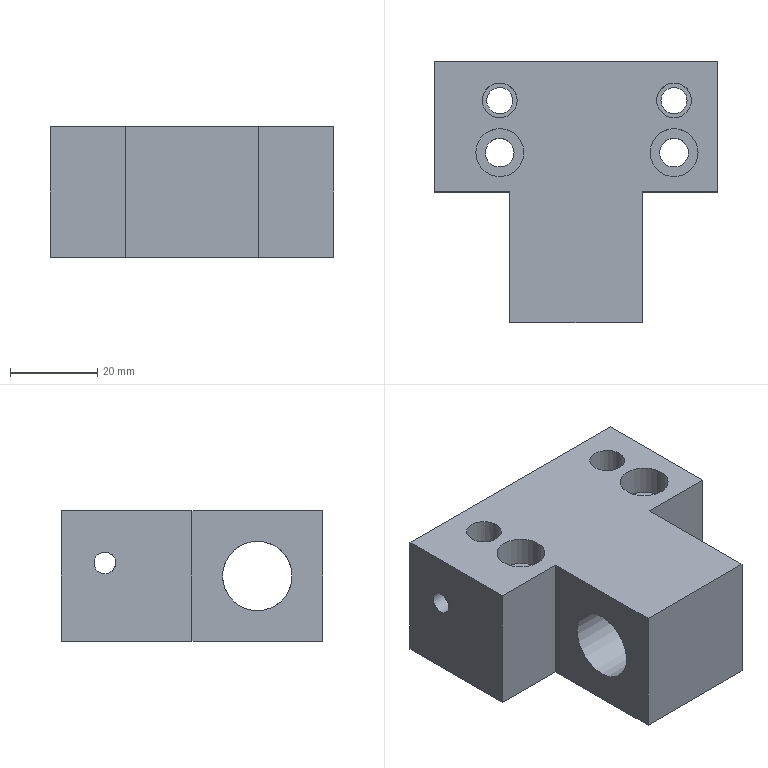Part | NX | features 5003_207_Bracket 2 | 1 solid | 26 faces | box 65 x 60 x 30 mm | volume 73364 mm3 | plane 14 | cylinder 12 | commonest cylinder face diameters 5 x3 6 x2 6.6 x2 8 x2 11 x2 16 x1
STEP:
#1=CARTESIAN_POINT('',(109.6,-462.,-238.));
#2=VERTEX_POINT('',#1);
#3=CARTESIAN_POINT('',(44.6,-462.,-238.));
#4=VERTEX_POINT('',#3);
#5=CARTESIAN_POINT('',(44.6,-462.,-238.));
#6=DIRECTION('',(-1.,0.,0.));
#7=VECTOR('',#6,1000.);
#8=LINE('',#5,#7);
#9=EDGE_CURVE('',#2,#4,#8,.T.);
#10=ORIENTED_EDGE('',*,*,#9,.T.);
#11=CARTESIAN_POINT('',(44.6,-462.,-208.));
#12=VERTEX_POINT('',#11);
#13=CARTESIAN_POINT('',(44.6,-462.,-208.));
#14=DIRECTION('',(0.,0.,-1.));
#15=VECTOR('',#14,1000.);
#16=LINE('',#13,#15);
#17=EDGE_CURVE('',#12,#4,#16,.T.);
#18=ORIENTED_EDGE('',*,*,#17,.F.);
#19=CARTESIAN_POINT('',(109.6,-462.,-208.));
#20=VERTEX_POINT('',#19);
#21=CARTESIAN_POINT('',(44.6,-462.,-208.));
#22=DIRECTION('',(-1.,0.,0.));
#23=VECTOR('',#22,1000.);
#24=LINE('',#21,#23);
#25=EDGE_CURVE('',#20,#12,#24,.T.);
#26=ORIENTED_EDGE('',*,*,#25,.F.);
#27=CARTESIAN_POINT('',(109.6,-462.,-208.));
#28=DIRECTION('',(0.,0.,-1.));
#29=VECTOR('',#28,1000.);
#30=LINE('',#27,#29);
#31=EDGE_CURVE('',#20,#2,#30,.T.);
#32=ORIENTED_EDGE('',*,*,#31,.T.);
#33=EDGE_LOOP('',(#10,#18,#26,#32));
#34=FACE_BOUND('',#33,.T.);
#35=CARTESIAN_POINT('',(44.6,-462.,-208.));
#36=DIRECTION('',(0.,-1.,0.));
#37=DIRECTION('',(1.,0.,0.));
#38=AXIS2_PLACEMENT_3D('',#35,#36,#37);
#39=PLANE('',#38);
#40=ADVANCED_FACE('',(#34),#39,.F.);
#41=CARTESIAN_POINT('',(44.6,-472.,-222.5));
#42=VERTEX_POINT('',#41);
#43=CARTESIAN_POINT('',(44.6,-472.,-220.));
#44=DIRECTION('',(-1.,0.,0.));
#45=DIRECTION('',(0.,0.,-1.));
#46=AXIS2_PLACEMENT_3D('',#43,#44,#45);
#47=CIRCLE('',#46,2.5);
#48=EDGE_CURVE('',#42,#42,#47,.T.);
#49=ORIENTED_EDGE('',*,*,#48,.F.);
#50=EDGE_LOOP('',(#49));
#51=FACE_BOUND('',#50,.T.);
#52=CARTESIAN_POINT('',(44.6,-492.,-238.));
#53=VERTEX_POINT('',#52);
#54=CARTESIAN_POINT('',(44.6,-492.,-238.));
#55=DIRECTION('',(0.,-1.,0.));
#56=VECTOR('',#55,1000.);
#57=LINE('',#54,#56);
#58=EDGE_CURVE('',#4,#53,#57,.T.);
#59=ORIENTED_EDGE('',*,*,#58,.T.);
#60=CARTESIAN_POINT('',(44.6,-492.,-208.));
#61=VERTEX_POINT('',#60);
#62=CARTESIAN_POINT('',(44.6,-492.,-208.));
#63=DIRECTION('',(0.,0.,-1.));
#64=VECTOR('',#63,1000.);
#65=LINE('',#62,#64);
#66=EDGE_CURVE('',#61,#53,#65,.T.);
#67=ORIENTED_EDGE('',*,*,#66,.F.);
#68=CARTESIAN_POINT('',(44.6,-492.,-208.));
#69=DIRECTION('',(0.,-1.,0.));
#70=VECTOR('',#69,1000.);
#71=LINE('',#68,#70);
#72=EDGE_CURVE('',#12,#61,#71,.T.);
#73=ORIENTED_EDGE('',*,*,#72,.F.);
#74=ORIENTED_EDGE('',*,*,#17,.T.);
#75=EDGE_LOOP('',(#59,#67,#73,#74));
#76=FACE_BOUND('',#75,.T.);
#77=CARTESIAN_POINT('',(44.6,-492.,-208.));
#78=DIRECTION('',(1.,0.,0.));
#79=DIRECTION('',(0.,0.,1.));
#80=AXIS2_PLACEMENT_3D('',#77,#78,#79);
#81=PLANE('',#80);
#82=ADVANCED_FACE('',(#51,#76),#81,.F.);
#83=CARTESIAN_POINT('',(61.855,-492.,-238.));
#84=VERTEX_POINT('',#83);
#85=CARTESIAN_POINT('',(61.855,-492.,-238.));
#86=DIRECTION('',(1.,0.,0.));
#87=VECTOR('',#86,1000.);
#88=LINE('',#85,#87);
#89=EDGE_CURVE('',#53,#84,#88,.T.);
#90=ORIENTED_EDGE('',*,*,#89,.T.);
#91=CARTESIAN_POINT('',(61.855,-492.,-208.));
#92=VERTEX_POINT('',#91);
#93=CARTESIAN_POINT('',(61.855,-492.,-208.));
#94=DIRECTION('',(0.,0.,-1.));
#95=VECTOR('',#94,1000.);
#96=LINE('',#93,#95);
#97=EDGE_CURVE('',#92,#84,#96,.T.);
#98=ORIENTED_EDGE('',*,*,#97,.F.);
#99=CARTESIAN_POINT('',(61.855,-492.,-208.));
#100=DIRECTION('',(1.,0.,0.));
#101=VECTOR('',#100,1000.);
#102=LINE('',#99,#101);
#103=EDGE_CURVE('',#61,#92,#102,.T.);
#104=ORIENTED_EDGE('',*,*,#103,.F.);
#105=ORIENTED_EDGE('',*,*,#66,.T.);
#106=EDGE_LOOP('',(#90,#98,#104,#105));
#107=FACE_BOUND('',#106,.T.);
#108=CARTESIAN_POINT('',(61.855,-492.,-208.));
#109=DIRECTION('',(0.,1.,0.));
#110=DIRECTION('',(-1.,0.,0.));
#111=AXIS2_PLACEMENT_3D('',#108,#109,#110);
#112=PLANE('',#111);
#113=ADVANCED_FACE('',(#107),#112,.F.);
#114=CARTESIAN_POINT('',(61.855,-507.,-231.));
#115=VERTEX_POINT('',#114);
#116=CARTESIAN_POINT('',(61.855,-507.,-223.));
#117=DIRECTION('',(-1.,0.,0.));
#118=DIRECTION('',(0.,0.,-1.));
#119=AXIS2_PLACEMENT_3D('',#116,#117,#118);
#120=CIRCLE('',#119,8.);
#121=EDGE_CURVE('',#115,#115,#120,.T.);
#122=ORIENTED_EDGE('',*,*,#121,.F.);
#123=EDGE_LOOP('',(#122));
#124=FACE_BOUND('',#123,.T.);
#125=CARTESIAN_POINT('',(61.855,-522.,-238.));
#126=VERTEX_POINT('',#125);
#127=CARTESIAN_POINT('',(61.855,-522.,-238.));
#128=DIRECTION('',(0.,-1.,0.));
#129=VECTOR('',#128,1000.);
#130=LINE('',#127,#129);
#131=EDGE_CURVE('',#84,#126,#130,.T.);
#132=ORIENTED_EDGE('',*,*,#131,.T.);
#133=CARTESIAN_POINT('',(61.855,-522.,-208.));
#134=VERTEX_POINT('',#133);
#135=CARTESIAN_POINT('',(61.855,-522.,-208.));
#136=DIRECTION('',(0.,0.,-1.));
#137=VECTOR('',#136,1000.);
#138=LINE('',#135,#137);
#139=EDGE_CURVE('',#134,#126,#138,.T.);
#140=ORIENTED_EDGE('',*,*,#139,.F.);
#141=CARTESIAN_POINT('',(61.855,-522.,-208.));
#142=DIRECTION('',(0.,-1.,0.));
#143=VECTOR('',#142,1000.);
#144=LINE('',#141,#143);
#145=EDGE_CURVE('',#92,#134,#144,.T.);
#146=ORIENTED_EDGE('',*,*,#145,.F.);
#147=ORIENTED_EDGE('',*,*,#97,.T.);
#148=EDGE_LOOP('',(#132,#140,#146,#147));
#149=FACE_BOUND('',#148,.T.);
#150=CARTESIAN_POINT('',(61.855,-522.,-208.));
#151=DIRECTION('',(1.,0.,0.));
#152=DIRECTION('',(0.,0.,1.));
#153=AXIS2_PLACEMENT_3D('',#150,#151,#152);
#154=PLANE('',#153);
#155=ADVANCED_FACE('',(#124,#149),#154,.F.);
#156=CARTESIAN_POINT('',(92.345,-522.,-238.));
#157=VERTEX_POINT('',#156);
#158=CARTESIAN_POINT('',(92.345,-522.,-238.));
#159=DIRECTION('',(1.,0.,0.));
#160=VECTOR('',#159,1000.);
#161=LINE('',#158,#160);
#162=EDGE_CURVE('',#126,#157,#161,.T.);
#163=ORIENTED_EDGE('',*,*,#162,.T.);
#164=CARTESIAN_POINT('',(92.345,-522.,-208.));
#165=VERTEX_POINT('',#164);
#166=CARTESIAN_POINT('',(92.345,-522.,-208.));
#167=DIRECTION('',(0.,0.,-1.));
#168=VECTOR('',#167,1000.);
#169=LINE('',#166,#168);
#170=EDGE_CURVE('',#165,#157,#169,.T.);
#171=ORIENTED_EDGE('',*,*,#170,.F.);
#172=CARTESIAN_POINT('',(92.345,-522.,-208.));
#173=DIRECTION('',(1.,0.,0.));
#174=VECTOR('',#173,1000.);
#175=LINE('',#172,#174);
#176=EDGE_CURVE('',#134,#165,#175,.T.);
#177=ORIENTED_EDGE('',*,*,#176,.F.);
#178=ORIENTED_EDGE('',*,*,#139,.T.);
#179=EDGE_LOOP('',(#163,#171,#177,#178));
#180=FACE_BOUND('',#179,.T.);
#181=CARTESIAN_POINT('',(92.345,-522.,-208.));
#182=DIRECTION('',(0.,1.,0.));
#183=DIRECTION('',(0.,0.,-1.));
#184=AXIS2_PLACEMENT_3D('',#181,#182,#183);
#185=PLANE('',#184);
#186=ADVANCED_FACE('',(#180),#185,.F.);
#187=CARTESIAN_POINT('',(92.345,-515.,-223.));
#188=VERTEX_POINT('',#187);
#189=CARTESIAN_POINT('',(92.345,-507.,-223.));
#190=DIRECTION('',(-1.,0.,0.));
#191=DIRECTION('',(0.,-1.,0.));
#192=AXIS2_PLACEMENT_3D('',#189,#190,#191);
#193=CIRCLE('',#192,8.);
#194=EDGE_CURVE('',#188,#188,#193,.T.);
#195=ORIENTED_EDGE('',*,*,#194,.T.);
#196=EDGE_LOOP('',(#195));
#197=FACE_BOUND('',#196,.T.);
#198=CARTESIAN_POINT('',(92.345,-492.,-238.));
#199=VERTEX_POINT('',#198);
#200=CARTESIAN_POINT('',(92.345,-492.,-238.));
#201=DIRECTION('',(0.,1.,0.));
#202=VECTOR('',#201,1000.);
#203=LINE('',#200,#202);
#204=EDGE_CURVE('',#157,#199,#203,.T.);
#205=ORIENTED_EDGE('',*,*,#204,.T.);
#206=CARTESIAN_POINT('',(92.345,-492.,-208.));
#207=VERTEX_POINT('',#206);
#208=CARTESIAN_POINT('',(92.345,-492.,-208.));
#209=DIRECTION('',(0.,0.,-1.));
#210=VECTOR('',#209,1000.);
#211=LINE('',#208,#210);
#212=EDGE_CURVE('',#207,#199,#211,.T.);
#213=ORIENTED_EDGE('',*,*,#212,.F.);
#214=CARTESIAN_POINT('',(92.345,-492.,-208.));
#215=DIRECTION('',(0.,1.,0.));
#216=VECTOR('',#215,1000.);
#217=LINE('',#214,#216);
#218=EDGE_CURVE('',#165,#207,#217,.T.);
#219=ORIENTED_EDGE('',*,*,#218,.F.);
#220=ORIENTED_EDGE('',*,*,#170,.T.);
#221=EDGE_LOOP('',(#205,#213,#219,#220));
#222=FACE_BOUND('',#221,.T.);
#223=CARTESIAN_POINT('',(92.345,-492.,-208.));
#224=DIRECTION('',(-1.,0.,0.));
#225=DIRECTION('',(0.,-1.,0.));
#226=AXIS2_PLACEMENT_3D('',#223,#224,#225);
#227=PLANE('',#226);
#228=ADVANCED_FACE('',(#197,#222),#227,.F.);
#229=CARTESIAN_POINT('',(109.6,-492.,-238.));
#230=VERTEX_POINT('',#229);
#231=CARTESIAN_POINT('',(109.6,-492.,-238.));
#232=DIRECTION('',(1.,0.,0.));
#233=VECTOR('',#232,1000.);
#234=LINE('',#231,#233);
#235=EDGE_CURVE('',#199,#230,#234,.T.);
#236=ORIENTED_EDGE('',*,*,#235,.T.);
#237=CARTESIAN_POINT('',(109.6,-492.,-208.));
#238=VERTEX_POINT('',#237);
#239=CARTESIAN_POINT('',(109.6,-492.,-208.));
#240=DIRECTION('',(0.,0.,-1.));
#241=VECTOR('',#240,1000.);
#242=LINE('',#239,#241);
#243=EDGE_CURVE('',#238,#230,#242,.T.);
#244=ORIENTED_EDGE('',*,*,#243,.F.);
#245=CARTESIAN_POINT('',(109.6,-492.,-208.));
#246=DIRECTION('',(1.,0.,0.));
#247=VECTOR('',#246,1000.);
#248=LINE('',#245,#247);
#249=EDGE_CURVE('',#207,#238,#248,.T.);
#250=ORIENTED_EDGE('',*,*,#249,.F.);
#251=ORIENTED_EDGE('',*,*,#212,.T.);
#252=EDGE_LOOP('',(#236,#244,#250,#251));
#253=FACE_BOUND('',#252,.T.);
#254=CARTESIAN_POINT('',(109.6,-492.,-208.));
#255=DIRECTION('',(0.,1.,0.));
#256=DIRECTION('',(0.,0.,-1.));
#257=AXIS2_PLACEMENT_3D('',#254,#255,#256);
#258=PLANE('',#257);
#259=ADVANCED_FACE('',(#253),#258,.F.);
#260=CARTESIAN_POINT('',(109.6,-472.,-222.5));
#261=VERTEX_POINT('',#260);
#262=CARTESIAN_POINT('',(109.6,-472.,-220.));
#263=DIRECTION('',(-1.,0.,0.));
#264=DIRECTION('',(0.,0.,-1.));
#265=AXIS2_PLACEMENT_3D('',#262,#263,#264);
#266=CIRCLE('',#265,2.5);
#267=EDGE_CURVE('',#261,#261,#266,.T.);
#268=ORIENTED_EDGE('',*,*,#267,.T.);
#269=EDGE_LOOP('',(#268));
#270=FACE_BOUND('',#269,.T.);
#271=CARTESIAN_POINT('',(109.6,-462.,-238.));
#272=DIRECTION('',(0.,1.,0.));
#273=VECTOR('',#272,1000.);
#274=LINE('',#271,#273);
#275=EDGE_CURVE('',#230,#2,#274,.T.);
#276=ORIENTED_EDGE('',*,*,#275,.T.);
#277=ORIENTED_EDGE('',*,*,#31,.F.);
#278=CARTESIAN_POINT('',(109.6,-462.,-208.));
#279=DIRECTION('',(0.,1.,0.));
#280=VECTOR('',#279,1000.);
#281=LINE('',#278,#280);
#282=EDGE_CURVE('',#238,#20,#281,.T.);
#283=ORIENTED_EDGE('',*,*,#282,.F.);
#284=ORIENTED_EDGE('',*,*,#243,.T.);
#285=EDGE_LOOP('',(#276,#277,#283,#284));
#286=FACE_BOUND('',#285,.T.);
#287=CARTESIAN_POINT('',(109.6,-462.,-208.));
#288=DIRECTION('',(-1.,0.,0.));
#289=DIRECTION('',(0.,-1.,0.));
#290=AXIS2_PLACEMENT_3D('',#287,#288,#289);
#291=PLANE('',#290);
#292=ADVANCED_FACE('',(#270,#286),#291,.F.);
#293=CARTESIAN_POINT('',(95.6,-471.,-208.));
#294=VERTEX_POINT('',#293);
#295=CARTESIAN_POINT('',(99.6,-471.,-208.));
#296=DIRECTION('',(0.,0.,1.));
#297=DIRECTION('',(-1.,0.,0.));
#298=AXIS2_PLACEMENT_3D('',#295,#296,#297);
#299=CIRCLE('',#298,4.);
#300=EDGE_CURVE('',#294,#294,#299,.T.);
#301=ORIENTED_EDGE('',*,*,#300,.F.);
#302=EDGE_LOOP('',(#301));
#303=FACE_BOUND('',#302,.T.);
#304=CARTESIAN_POINT('',(55.6,-471.,-208.));
#305=VERTEX_POINT('',#304);
#306=CARTESIAN_POINT('',(59.6,-471.,-208.));
#307=DIRECTION('',(0.,0.,1.));
#308=DIRECTION('',(-1.,0.,0.));
#309=AXIS2_PLACEMENT_3D('',#306,#307,#308);
#310=CIRCLE('',#309,4.);
#311=EDGE_CURVE('',#305,#305,#310,.T.);
#312=ORIENTED_EDGE('',*,*,#311,.F.);
#313=EDGE_LOOP('',(#312));
#314=FACE_BOUND('',#313,.T.);
#315=CARTESIAN_POINT('',(94.1,-483.,-208.));
#316=VERTEX_POINT('',#315);
#317=CARTESIAN_POINT('',(99.6,-483.,-208.));
#318=DIRECTION('',(0.,0.,1.));
#319=DIRECTION('',(-1.,0.,0.));
#320=AXIS2_PLACEMENT_3D('',#317,#318,#319);
#321=CIRCLE('',#320,5.5);
#322=EDGE_CURVE('',#316,#316,#321,.T.);
#323=ORIENTED_EDGE('',*,*,#322,.F.);
#324=EDGE_LOOP('',(#323));
#325=FACE_BOUND('',#324,.T.);
#326=CARTESIAN_POINT('',(54.1,-483.,-208.));
#327=VERTEX_POINT('',#326);
#328=CARTESIAN_POINT('',(59.6,-483.,-208.));
#329=DIRECTION('',(0.,0.,1.));
#330=DIRECTION('',(-1.,0.,0.));
#331=AXIS2_PLACEMENT_3D('',#328,#329,#330);
#332=CIRCLE('',#331,5.5);
#333=EDGE_CURVE('',#327,#327,#332,.T.);
#334=ORIENTED_EDGE('',*,*,#333,.F.);
#335=EDGE_LOOP('',(#334));
#336=FACE_BOUND('',#335,.T.);
#337=ORIENTED_EDGE('',*,*,#25,.T.);
#338=ORIENTED_EDGE('',*,*,#72,.T.);
#339=ORIENTED_EDGE('',*,*,#103,.T.);
#340=ORIENTED_EDGE('',*,*,#145,.T.);
#341=ORIENTED_EDGE('',*,*,#176,.T.);
#342=ORIENTED_EDGE('',*,*,#218,.T.);
#343=ORIENTED_EDGE('',*,*,#249,.T.);
#344=ORIENTED_EDGE('',*,*,#282,.T.);
#345=EDGE_LOOP('',(#337,#338,#339,#340,#341,#342,#343,#344));
#346=FACE_BOUND('',#345,.T.);
#347=CARTESIAN_POINT('',(109.6,-462.,-208.));
#348=DIRECTION('',(0.,0.,-1.));
#349=DIRECTION('',(1.,0.,0.));
#350=AXIS2_PLACEMENT_3D('',#347,#348,#349);
#351=PLANE('',#350);
#352=ADVANCED_FACE('',(#303,#314,#325,#336,#346),#351,.F.);
#353=CARTESIAN_POINT('',(96.6,-471.,-238.));
#354=VERTEX_POINT('',#353);
#355=CARTESIAN_POINT('',(99.6,-471.,-238.));
#356=DIRECTION('',(0.,0.,1.));
#357=DIRECTION('',(-1.,0.,0.));
#358=AXIS2_PLACEMENT_3D('',#355,#356,#357);
#359=CIRCLE('',#358,3.);
#360=EDGE_CURVE('',#354,#354,#359,.T.);
#361=ORIENTED_EDGE('',*,*,#360,.T.);
#362=EDGE_LOOP('',(#361));
#363=FACE_BOUND('',#362,.T.);
#364=CARTESIAN_POINT('',(56.6,-471.,-238.));
#365=VERTEX_POINT('',#364);
#366=CARTESIAN_POINT('',(59.6,-471.,-238.));
#367=DIRECTION('',(0.,0.,1.));
#368=DIRECTION('',(-1.,0.,0.));
#369=AXIS2_PLACEMENT_3D('',#366,#367,#368);
#370=CIRCLE('',#369,3.);
#371=EDGE_CURVE('',#365,#365,#370,.T.);
#372=ORIENTED_EDGE('',*,*,#371,.T.);
#373=EDGE_LOOP('',(#372));
#374=FACE_BOUND('',#373,.T.);
#375=CARTESIAN_POINT('',(96.3,-483.,-238.));
#376=VERTEX_POINT('',#375);
#377=CARTESIAN_POINT('',(99.6,-483.,-238.));
#378=DIRECTION('',(0.,0.,1.));
#379=DIRECTION('',(-1.,0.,0.));
#380=AXIS2_PLACEMENT_3D('',#377,#378,#379);
#381=CIRCLE('',#380,3.3);
#382=EDGE_CURVE('',#376,#376,#381,.T.);
#383=ORIENTED_EDGE('',*,*,#382,.T.);
#384=EDGE_LOOP('',(#383));
#385=FACE_BOUND('',#384,.T.);
#386=CARTESIAN_POINT('',(56.3,-483.,-238.));
#387=VERTEX_POINT('',#386);
#388=CARTESIAN_POINT('',(59.6,-483.,-238.));
#389=DIRECTION('',(0.,0.,1.));
#390=DIRECTION('',(-1.,0.,0.));
#391=AXIS2_PLACEMENT_3D('',#388,#389,#390);
#392=CIRCLE('',#391,3.3);
#393=EDGE_CURVE('',#387,#387,#392,.T.);
#394=ORIENTED_EDGE('',*,*,#393,.T.);
#395=EDGE_LOOP('',(#394));
#396=FACE_BOUND('',#395,.T.);
#397=ORIENTED_EDGE('',*,*,#9,.F.);
#398=ORIENTED_EDGE('',*,*,#275,.F.);
#399=ORIENTED_EDGE('',*,*,#235,.F.);
#400=ORIENTED_EDGE('',*,*,#204,.F.);
#401=ORIENTED_EDGE('',*,*,#162,.F.);
#402=ORIENTED_EDGE('',*,*,#131,.F.);
#403=ORIENTED_EDGE('',*,*,#89,.F.);
#404=ORIENTED_EDGE('',*,*,#58,.F.);
#405=EDGE_LOOP('',(#397,#398,#399,#400,#401,#402,#403,#404));
#406=FACE_BOUND('',#405,.T.);
#407=CARTESIAN_POINT('',(109.6,-462.,-238.));
#408=DIRECTION('',(0.,0.,-1.));
#409=DIRECTION('',(1.,0.,0.));
#410=AXIS2_PLACEMENT_3D('',#407,#408,#409);
#411=PLANE('',#410);
#412=ADVANCED_FACE('',(#363,#374,#385,#396,#406),#411,.T.);
#413=ORIENTED_EDGE('',*,*,#393,.F.);
#414=EDGE_LOOP('',(#413));
#415=FACE_BOUND('',#414,.T.);
#416=CARTESIAN_POINT('',(56.3,-483.,-214.8));
#417=VERTEX_POINT('',#416);
#418=CARTESIAN_POINT('',(59.6,-483.,-214.8));
#419=DIRECTION('',(0.,0.,1.));
#420=DIRECTION('',(-1.,0.,0.));
#421=AXIS2_PLACEMENT_3D('',#418,#419,#420);
#422=CIRCLE('',#421,3.3);
#423=EDGE_CURVE('',#417,#417,#422,.T.);
#424=ORIENTED_EDGE('',*,*,#423,.T.);
#425=EDGE_LOOP('',(#424));
#426=FACE_BOUND('',#425,.T.);
#427=CARTESIAN_POINT('',(59.6,-483.,-208.));
#428=DIRECTION('',(0.,0.,1.));
#429=DIRECTION('',(-1.,0.,0.));
#430=AXIS2_PLACEMENT_3D('',#427,#428,#429);
#431=CYLINDRICAL_SURFACE('',#430,3.3);
#432=ADVANCED_FACE('',(#415,#426),#431,.F.);
#433=ORIENTED_EDGE('',*,*,#423,.F.);
#434=EDGE_LOOP('',(#433));
#435=FACE_BOUND('',#434,.T.);
#436=CARTESIAN_POINT('',(54.1,-483.,-214.8));
#437=VERTEX_POINT('',#436);
#438=CARTESIAN_POINT('',(59.6,-483.,-214.8));
#439=DIRECTION('',(0.,0.,1.));
#440=DIRECTION('',(-1.,0.,0.));
#441=AXIS2_PLACEMENT_3D('',#438,#439,#440);
#442=CIRCLE('',#441,5.5);
#443=EDGE_CURVE('',#437,#437,#442,.T.);
#444=ORIENTED_EDGE('',*,*,#443,.T.);
#445=EDGE_LOOP('',(#444));
#446=FACE_BOUND('',#445,.T.);
#447=CARTESIAN_POINT('',(56.3,-483.,-214.8));
#448=DIRECTION('',(0.,0.,-1.));
#449=DIRECTION('',(1.,0.,0.));
#450=AXIS2_PLACEMENT_3D('',#447,#448,#449);
#451=PLANE('',#450);
#452=ADVANCED_FACE('',(#435,#446),#451,.F.);
#453=ORIENTED_EDGE('',*,*,#443,.F.);
#454=EDGE_LOOP('',(#453));
#455=FACE_BOUND('',#454,.T.);
#456=ORIENTED_EDGE('',*,*,#333,.T.);
#457=EDGE_LOOP('',(#456));
#458=FACE_BOUND('',#457,.T.);
#459=CARTESIAN_POINT('',(59.6,-483.,-208.));
#460=DIRECTION('',(0.,0.,1.));
#461=DIRECTION('',(-1.,0.,0.));
#462=AXIS2_PLACEMENT_3D('',#459,#460,#461);
#463=CYLINDRICAL_SURFACE('',#462,5.5);
#464=ADVANCED_FACE('',(#455,#458),#463,.F.);
#465=ORIENTED_EDGE('',*,*,#382,.F.);
#466=EDGE_LOOP('',(#465));
#467=FACE_BOUND('',#466,.T.);
#468=CARTESIAN_POINT('',(96.3,-483.,-214.8));
#469=VERTEX_POINT('',#468);
#470=CARTESIAN_POINT('',(99.6,-483.,-214.8));
#471=DIRECTION('',(0.,0.,1.));
#472=DIRECTION('',(-1.,0.,0.));
#473=AXIS2_PLACEMENT_3D('',#470,#471,#472);
#474=CIRCLE('',#473,3.3);
#475=EDGE_CURVE('',#469,#469,#474,.T.);
#476=ORIENTED_EDGE('',*,*,#475,.T.);
#477=EDGE_LOOP('',(#476));
#478=FACE_BOUND('',#477,.T.);
#479=CARTESIAN_POINT('',(99.6,-483.,-208.));
#480=DIRECTION('',(0.,0.,1.));
#481=DIRECTION('',(-1.,0.,0.));
#482=AXIS2_PLACEMENT_3D('',#479,#480,#481);
#483=CYLINDRICAL_SURFACE('',#482,3.3);
#484=ADVANCED_FACE('',(#467,#478),#483,.F.);
#485=ORIENTED_EDGE('',*,*,#475,.F.);
#486=EDGE_LOOP('',(#485));
#487=FACE_BOUND('',#486,.T.);
#488=CARTESIAN_POINT('',(94.1,-483.,-214.8));
#489=VERTEX_POINT('',#488);
#490=CARTESIAN_POINT('',(99.6,-483.,-214.8));
#491=DIRECTION('',(0.,0.,1.));
#492=DIRECTION('',(-1.,0.,0.));
#493=AXIS2_PLACEMENT_3D('',#490,#491,#492);
#494=CIRCLE('',#493,5.5);
#495=EDGE_CURVE('',#489,#489,#494,.T.);
#496=ORIENTED_EDGE('',*,*,#495,.T.);
#497=EDGE_LOOP('',(#496));
#498=FACE_BOUND('',#497,.T.);
#499=CARTESIAN_POINT('',(96.3,-483.,-214.8));
#500=DIRECTION('',(0.,0.,-1.));
#501=DIRECTION('',(1.,0.,0.));
#502=AXIS2_PLACEMENT_3D('',#499,#500,#501);
#503=PLANE('',#502);
#504=ADVANCED_FACE('',(#487,#498),#503,.F.);
#505=ORIENTED_EDGE('',*,*,#495,.F.);
#506=EDGE_LOOP('',(#505));
#507=FACE_BOUND('',#506,.T.);
#508=ORIENTED_EDGE('',*,*,#322,.T.);
#509=EDGE_LOOP('',(#508));
#510=FACE_BOUND('',#509,.T.);
#511=CARTESIAN_POINT('',(99.6,-483.,-208.));
#512=DIRECTION('',(0.,0.,1.));
#513=DIRECTION('',(-1.,0.,0.));
#514=AXIS2_PLACEMENT_3D('',#511,#512,#513);
#515=CYLINDRICAL_SURFACE('',#514,5.5);
#516=ADVANCED_FACE('',(#507,#510),#515,.F.);
#517=ORIENTED_EDGE('',*,*,#371,.F.);
#518=EDGE_LOOP('',(#517));
#519=FACE_BOUND('',#518,.T.);
#520=CARTESIAN_POINT('',(56.6,-471.,-228.));
#521=VERTEX_POINT('',#520);
#522=CARTESIAN_POINT('',(59.6,-471.,-228.));
#523=DIRECTION('',(0.,0.,1.));
#524=DIRECTION('',(-1.,0.,0.));
#525=AXIS2_PLACEMENT_3D('',#522,#523,#524);
#526=CIRCLE('',#525,3.);
#527=EDGE_CURVE('',#521,#521,#526,.T.);
#528=ORIENTED_EDGE('',*,*,#527,.T.);
#529=EDGE_LOOP('',(#528));
#530=FACE_BOUND('',#529,.T.);
#531=CARTESIAN_POINT('',(59.6,-471.,-208.));
#532=DIRECTION('',(0.,0.,1.));
#533=DIRECTION('',(-1.,0.,0.));
#534=AXIS2_PLACEMENT_3D('',#531,#532,#533);
#535=CYLINDRICAL_SURFACE('',#534,3.);
#536=ADVANCED_FACE('',(#519,#530),#535,.F.);
#537=ORIENTED_EDGE('',*,*,#527,.F.);
#538=EDGE_LOOP('',(#537));
#539=FACE_BOUND('',#538,.T.);
#540=CARTESIAN_POINT('',(55.6,-471.,-228.));
#541=VERTEX_POINT('',#540);
#542=CARTESIAN_POINT('',(59.6,-471.,-228.));
#543=DIRECTION('',(0.,0.,1.));
#544=DIRECTION('',(-1.,0.,0.));
#545=AXIS2_PLACEMENT_3D('',#542,#543,#544);
#546=CIRCLE('',#545,4.);
#547=EDGE_CURVE('',#541,#541,#546,.T.);
#548=ORIENTED_EDGE('',*,*,#547,.T.);
#549=EDGE_LOOP('',(#548));
#550=FACE_BOUND('',#549,.T.);
#551=CARTESIAN_POINT('',(56.6,-471.,-228.));
#552=DIRECTION('',(0.,0.,-1.));
#553=DIRECTION('',(1.,0.,0.));
#554=AXIS2_PLACEMENT_3D('',#551,#552,#553);
#555=PLANE('',#554);
#556=ADVANCED_FACE('',(#539,#550),#555,.F.);
#557=CARTESIAN_POINT('',(55.6,-471.,-222.291));
#558=VERTEX_POINT('',#557);
#559=CARTESIAN_POINT('',(55.947,-469.346,-220.906));
#560=CARTESIAN_POINT('',(55.516,-470.615,-222.29));
#561=CARTESIAN_POINT('',(55.684,-472.023,-222.571));
#562=CARTESIAN_POINT('',(56.085,-472.995,-222.357));
#563=CARTESIAN_POINT('',(56.648,-473.744,-221.858));
#564=CARTESIAN_POINT('',(57.246,-474.262,-221.182));
#565=CARTESIAN_POINT('',(57.78,-474.564,-220.245));
#566=CARTESIAN_POINT('',(57.51,-474.424,-219.165));
#567=CARTESIAN_POINT('',(56.901,-473.991,-218.415));
#568=CARTESIAN_POINT('',(56.315,-473.344,-217.828));
#569=CARTESIAN_POINT('',(55.828,-472.463,-217.477));
#570=CARTESIAN_POINT('',(55.487,-471.062,-217.497));
#571=CARTESIAN_POINT('',(55.829,-469.543,-218.636));
#572=CARTESIAN_POINT('',(55.947,-469.346,-220.906));
#573=CARTESIAN_POINT('',(55.516,-470.615,-222.29));
#574=CARTESIAN_POINT('',(55.684,-472.023,-222.571));
#575=B_SPLINE_CURVE_WITH_KNOTS('',3,(#559,#560,#561,#562,#563,#564,#565,#566,#567,#568,#569,#570,#571,#572,#573,#574),.UNSPECIFIED.,.T.,.F.,(1,1,1,1,1,1,1,1,1,1,1,1,1,1,1,1,1,1,1,1),(-0.006259,-0.004173,-0.002086,0.,0.001043,0.002086,0.003129,0.004173,0.005216,0.006259,0.007302,0.008345,0.009388,0.01043,0.01252,0.0146,0.01669,0.01773,0.01878,0.01982),.UNSPECIFIED.);
#576=EDGE_CURVE('',#558,#558,#575,.T.);
#577=ORIENTED_EDGE('',*,*,#576,.T.);
#578=EDGE_LOOP('',(#577));
#579=FACE_BOUND('',#578,.T.);
#580=CARTESIAN_POINT('',(63.473,-472.,-222.5));
#581=VERTEX_POINT('',#580);
#582=CARTESIAN_POINT('',(63.118,-472.99,-222.359));
#583=CARTESIAN_POINT('',(63.52,-472.012,-222.571));
#584=CARTESIAN_POINT('',(63.642,-470.962,-222.356));
#585=CARTESIAN_POINT('',(63.474,-469.808,-221.528));
#586=CARTESIAN_POINT('',(63.17,-469.209,-219.738));
#587=CARTESIAN_POINT('',(63.581,-470.119,-218.1));
#588=CARTESIAN_POINT('',(63.625,-471.418,-217.493));
#589=CARTESIAN_POINT('',(63.373,-472.465,-217.477));
#590=CARTESIAN_POINT('',(62.884,-473.348,-217.83));
#591=CARTESIAN_POINT('',(62.295,-473.996,-218.421));
#592=CARTESIAN_POINT('',(61.684,-474.428,-219.174));
#593=CARTESIAN_POINT('',(61.424,-474.562,-220.261));
#594=CARTESIAN_POINT('',(61.962,-474.257,-221.19));
#595=CARTESIAN_POINT('',(62.56,-473.736,-221.865));
#596=CARTESIAN_POINT('',(63.118,-472.99,-222.359));
#597=CARTESIAN_POINT('',(63.52,-472.012,-222.571));
#598=CARTESIAN_POINT('',(63.642,-470.962,-222.356));
#599=B_SPLINE_CURVE_WITH_KNOTS('',3,(#582,#583,#584,#585,#586,#587,#588,#589,#590,#591,#592,#593,#594,#595,#596,#597,#598),.UNSPECIFIED.,.T.,.F.,(1,1,1,1,1,1,1,1,1,1,1,1,1,1,1,1,1,1,1,1,1),(-0.003125,-0.002084,-0.001042,0.,0.001042,0.002084,0.004167,0.006251,0.007293,0.008335,0.009376,0.01042,0.01146,0.0125,0.01354,0.01459,0.01563,0.01667,0.01771,0.01875,0.02084),.UNSPECIFIED.);
#600=EDGE_CURVE('',#581,#581,#599,.T.);
#601=ORIENTED_EDGE('',*,*,#600,.T.);
#602=EDGE_LOOP('',(#601));
#603=FACE_BOUND('',#602,.T.);
#604=ORIENTED_EDGE('',*,*,#547,.F.);
#605=EDGE_LOOP('',(#604));
#606=FACE_BOUND('',#605,.T.);
#607=ORIENTED_EDGE('',*,*,#311,.T.);
#608=EDGE_LOOP('',(#607));
#609=FACE_BOUND('',#608,.T.);
#610=CARTESIAN_POINT('',(59.6,-471.,-208.));
#611=DIRECTION('',(0.,0.,1.));
#612=DIRECTION('',(-1.,0.,0.));
#613=AXIS2_PLACEMENT_3D('',#610,#611,#612);
#614=CYLINDRICAL_SURFACE('',#613,4.);
#615=ADVANCED_FACE('',(#579,#603,#606,#609),#614,.F.);
#616=ORIENTED_EDGE('',*,*,#360,.F.);
#617=EDGE_LOOP('',(#616));
#618=FACE_BOUND('',#617,.T.);
#619=CARTESIAN_POINT('',(96.6,-471.,-228.));
#620=VERTEX_POINT('',#619);
#621=CARTESIAN_POINT('',(99.6,-471.,-228.));
#622=DIRECTION('',(0.,0.,1.));
#623=DIRECTION('',(-1.,0.,0.));
#624=AXIS2_PLACEMENT_3D('',#621,#622,#623);
#625=CIRCLE('',#624,3.);
#626=EDGE_CURVE('',#620,#620,#625,.T.);
#627=ORIENTED_EDGE('',*,*,#626,.T.);
#628=EDGE_LOOP('',(#627));
#629=FACE_BOUND('',#628,.T.);
#630=CARTESIAN_POINT('',(99.6,-471.,-208.));
#631=DIRECTION('',(0.,0.,1.));
#632=DIRECTION('',(-1.,0.,0.));
#633=AXIS2_PLACEMENT_3D('',#630,#631,#632);
#634=CYLINDRICAL_SURFACE('',#633,3.);
#635=ADVANCED_FACE('',(#618,#629),#634,.F.);
#636=ORIENTED_EDGE('',*,*,#626,.F.);
#637=EDGE_LOOP('',(#636));
#638=FACE_BOUND('',#637,.T.);
#639=CARTESIAN_POINT('',(95.6,-471.,-228.));
#640=VERTEX_POINT('',#639);
#641=CARTESIAN_POINT('',(99.6,-471.,-228.));
#642=DIRECTION('',(0.,0.,1.));
#643=DIRECTION('',(-1.,0.,0.));
#644=AXIS2_PLACEMENT_3D('',#641,#642,#643);
#645=CIRCLE('',#644,4.);
#646=EDGE_CURVE('',#640,#640,#645,.T.);
#647=ORIENTED_EDGE('',*,*,#646,.T.);
#648=EDGE_LOOP('',(#647));
#649=FACE_BOUND('',#648,.T.);
#650=CARTESIAN_POINT('',(96.6,-471.,-228.));
#651=DIRECTION('',(0.,0.,-1.));
#652=DIRECTION('',(1.,0.,0.));
#653=AXIS2_PLACEMENT_3D('',#650,#651,#652);
#654=PLANE('',#653);
#655=ADVANCED_FACE('',(#638,#649),#654,.F.);
#656=CARTESIAN_POINT('',(95.6,-471.,-222.291));
#657=VERTEX_POINT('',#656);
#658=CARTESIAN_POINT('',(95.947,-469.346,-220.906));
#659=CARTESIAN_POINT('',(95.516,-470.615,-222.29));
#660=CARTESIAN_POINT('',(95.684,-472.023,-222.571));
#661=CARTESIAN_POINT('',(96.085,-472.995,-222.357));
#662=CARTESIAN_POINT('',(96.648,-473.744,-221.858));
#663=CARTESIAN_POINT('',(97.246,-474.262,-221.182));
#664=CARTESIAN_POINT('',(97.78,-474.564,-220.245));
#665=CARTESIAN_POINT('',(97.51,-474.424,-219.165));
#666=CARTESIAN_POINT('',(96.901,-473.991,-218.415));
#667=CARTESIAN_POINT('',(96.315,-473.344,-217.828));
#668=CARTESIAN_POINT('',(95.828,-472.463,-217.477));
#669=CARTESIAN_POINT('',(95.487,-471.062,-217.497));
#670=CARTESIAN_POINT('',(95.829,-469.543,-218.636));
#671=CARTESIAN_POINT('',(95.947,-469.346,-220.906));
#672=CARTESIAN_POINT('',(95.516,-470.615,-222.29));
#673=CARTESIAN_POINT('',(95.684,-472.023,-222.571));
#674=B_SPLINE_CURVE_WITH_KNOTS('',3,(#658,#659,#660,#661,#662,#663,#664,#665,#666,#667,#668,#669,#670,#671,#672,#673),.UNSPECIFIED.,.T.,.F.,(1,1,1,1,1,1,1,1,1,1,1,1,1,1,1,1,1,1,1,1),(-0.006259,-0.004173,-0.002086,0.,0.001043,0.002086,0.003129,0.004173,0.005216,0.006259,0.007302,0.008345,0.009388,0.01043,0.01252,0.0146,0.01669,0.01773,0.01878,0.01982),.UNSPECIFIED.);
#675=EDGE_CURVE('',#657,#657,#674,.T.);
#676=ORIENTED_EDGE('',*,*,#675,.T.);
#677=EDGE_LOOP('',(#676));
#678=FACE_BOUND('',#677,.T.);
#679=CARTESIAN_POINT('',(103.473,-472.,-222.5));
#680=VERTEX_POINT('',#679);
#681=CARTESIAN_POINT('',(103.118,-472.99,-222.359));
#682=CARTESIAN_POINT('',(103.52,-472.012,-222.571));
#683=CARTESIAN_POINT('',(103.642,-470.962,-222.356));
#684=CARTESIAN_POINT('',(103.474,-469.808,-221.528));
#685=CARTESIAN_POINT('',(103.17,-469.209,-219.738));
#686=CARTESIAN_POINT('',(103.581,-470.119,-218.1));
#687=CARTESIAN_POINT('',(103.625,-471.418,-217.493));
#688=CARTESIAN_POINT('',(103.373,-472.465,-217.477));
#689=CARTESIAN_POINT('',(102.884,-473.348,-217.83));
#690=CARTESIAN_POINT('',(102.295,-473.996,-218.421));
#691=CARTESIAN_POINT('',(101.684,-474.428,-219.174));
#692=CARTESIAN_POINT('',(101.424,-474.562,-220.261));
#693=CARTESIAN_POINT('',(101.962,-474.257,-221.19));
#694=CARTESIAN_POINT('',(102.56,-473.736,-221.865));
#695=CARTESIAN_POINT('',(103.118,-472.99,-222.359));
#696=CARTESIAN_POINT('',(103.52,-472.012,-222.571));
#697=CARTESIAN_POINT('',(103.642,-470.962,-222.356));
#698=B_SPLINE_CURVE_WITH_KNOTS('',3,(#681,#682,#683,#684,#685,#686,#687,#688,#689,#690,#691,#692,#693,#694,#695,#696,#697),.UNSPECIFIED.,.T.,.F.,(1,1,1,1,1,1,1,1,1,1,1,1,1,1,1,1,1,1,1,1,1),(-0.003125,-0.002084,-0.001042,0.,0.001042,0.002084,0.004167,0.006251,0.007293,0.008335,0.009376,0.01042,0.01146,0.0125,0.01354,0.01459,0.01563,0.01667,0.01771,0.01875,0.02084),.UNSPECIFIED.);
#699=EDGE_CURVE('',#680,#680,#698,.T.);
#700=ORIENTED_EDGE('',*,*,#699,.T.);
#701=EDGE_LOOP('',(#700));
#702=FACE_BOUND('',#701,.T.);
#703=ORIENTED_EDGE('',*,*,#646,.F.);
#704=EDGE_LOOP('',(#703));
#705=FACE_BOUND('',#704,.T.);
#706=ORIENTED_EDGE('',*,*,#300,.T.);
#707=EDGE_LOOP('',(#706));
#708=FACE_BOUND('',#707,.T.);
#709=CARTESIAN_POINT('',(99.6,-471.,-208.));
#710=DIRECTION('',(0.,0.,1.));
#711=DIRECTION('',(-1.,0.,0.));
#712=AXIS2_PLACEMENT_3D('',#709,#710,#711);
#713=CYLINDRICAL_SURFACE('',#712,4.);
#714=ADVANCED_FACE('',(#678,#702,#705,#708),#713,.F.);
#715=ORIENTED_EDGE('',*,*,#600,.F.);
#716=EDGE_LOOP('',(#715));
#717=FACE_BOUND('',#716,.T.);
#718=ORIENTED_EDGE('',*,*,#675,.F.);
#719=EDGE_LOOP('',(#718));
#720=FACE_BOUND('',#719,.T.);
#721=CARTESIAN_POINT('',(44.6,-472.,-220.));
#722=DIRECTION('',(-1.,0.,0.));
#723=DIRECTION('',(0.,0.,-1.));
#724=AXIS2_PLACEMENT_3D('',#721,#722,#723);
#725=CYLINDRICAL_SURFACE('',#724,2.5);
#726=ADVANCED_FACE('',(#717,#720),#725,.F.);
#727=ORIENTED_EDGE('',*,*,#267,.F.);
#728=EDGE_LOOP('',(#727));
#729=FACE_BOUND('',#728,.T.);
#730=ORIENTED_EDGE('',*,*,#699,.F.);
#731=EDGE_LOOP('',(#730));
#732=FACE_BOUND('',#731,.T.);
#733=CARTESIAN_POINT('',(44.6,-472.,-220.));
#734=DIRECTION('',(-1.,0.,0.));
#735=DIRECTION('',(0.,0.,-1.));
#736=AXIS2_PLACEMENT_3D('',#733,#734,#735);
#737=CYLINDRICAL_SURFACE('',#736,2.5);
#738=ADVANCED_FACE('',(#729,#732),#737,.F.);
#739=ORIENTED_EDGE('',*,*,#48,.T.);
#740=EDGE_LOOP('',(#739));
#741=FACE_BOUND('',#740,.T.);
#742=ORIENTED_EDGE('',*,*,#576,.F.);
#743=EDGE_LOOP('',(#742));
#744=FACE_BOUND('',#743,.T.);
#745=CARTESIAN_POINT('',(44.6,-472.,-220.));
#746=DIRECTION('',(-1.,0.,0.));
#747=DIRECTION('',(0.,0.,-1.));
#748=AXIS2_PLACEMENT_3D('',#745,#746,#747);
#749=CYLINDRICAL_SURFACE('',#748,2.5);
#750=ADVANCED_FACE('',(#741,#744),#749,.F.);
#751=ORIENTED_EDGE('',*,*,#121,.T.);
#752=EDGE_LOOP('',(#751));
#753=FACE_BOUND('',#752,.T.);
#754=ORIENTED_EDGE('',*,*,#194,.F.);
#755=EDGE_LOOP('',(#754));
#756=FACE_BOUND('',#755,.T.);
#757=CARTESIAN_POINT('',(61.855,-507.,-223.));
#758=DIRECTION('',(-1.,0.,0.));
#759=DIRECTION('',(0.,0.,-1.));
#760=AXIS2_PLACEMENT_3D('',#757,#758,#759);
#761=CYLINDRICAL_SURFACE('',#760,8.);
#762=ADVANCED_FACE('',(#753,#756),#761,.F.);
#763=CLOSED_SHELL('',(#40,#82,#113,#155,#186,#228,#259,#292,#352,#412,#432,#452,#464,#484,#504,#516,#536,#556,#615,#635,#655,#714,#726,#738,#750,#762));
#764=MANIFOLD_SOLID_BREP('',#763);
#765=(LENGTH_UNIT()NAMED_UNIT(*)SI_UNIT(.MILLI.,.METRE.));
#766=UNCERTAINTY_MEASURE_WITH_UNIT(LENGTH_MEASURE(0.0508),#765,'','');
#767=(NAMED_UNIT(*)PLANE_ANGLE_UNIT()SI_UNIT($,.RADIAN.));
#768=(NAMED_UNIT(*)SI_UNIT($,.STERADIAN.)SOLID_ANGLE_UNIT());
#769=(GEOMETRIC_REPRESENTATION_CONTEXT(3)GLOBAL_UNCERTAINTY_ASSIGNED_CONTEXT((#766))GLOBAL_UNIT_ASSIGNED_CONTEXT((#765,#767,#768))REPRESENTATION_CONTEXT('',''));
#770=ADVANCED_BREP_SHAPE_REPRESENTATION('',(#764),#769);